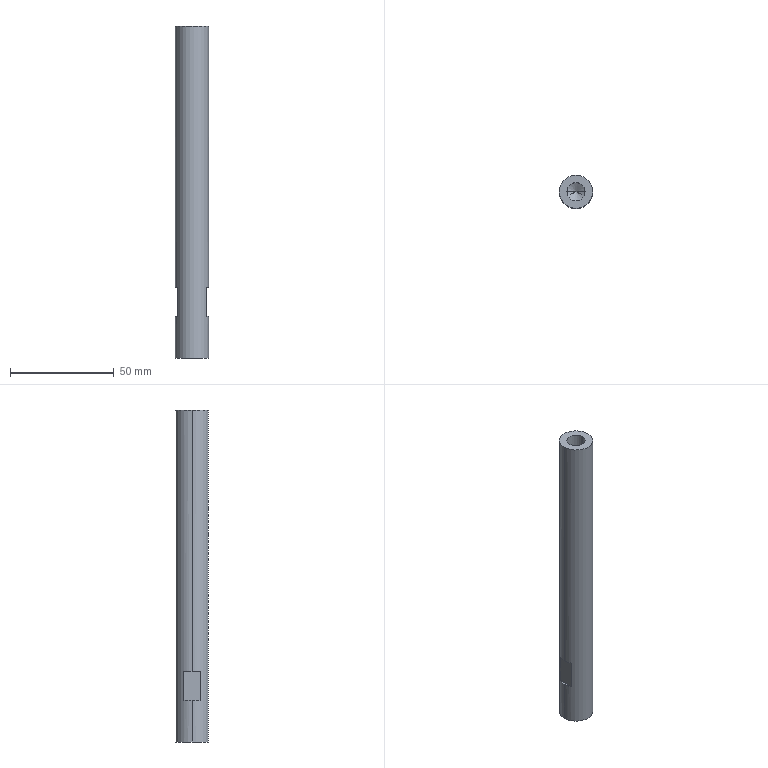Part | STEP file | Guide pillar | 1 solid | 18 faces | box 16 x 16 x 160 mm | volume 28723 mm3 | plane 8 | cylinder 6 | cone 4 | commonest cylinder face diameters 8.8 x4 16 x2
STEP:
#1=CARTESIAN_POINT('',(0.,0.,0.));
#2=DIRECTION('',(0.,0.,1.));
#3=DIRECTION('',(1.,0.,0.));
#4=AXIS2_PLACEMENT_3D('',#1,#2,#3);
#5=CARTESIAN_POINT('',(-4.4,0.,26.25));
#6=VERTEX_POINT('',#5);
#7=CARTESIAN_POINT('',(-4.4,0.,0.));
#8=VERTEX_POINT('',#7);
#9=CARTESIAN_POINT('',(-4.4,0.,0.));
#10=DIRECTION('',(0.,0.,-1.));
#11=VECTOR('',#10,1.);
#12=LINE('',#9,#11);
#13=CARTESIAN_POINT('',(0.,0.,0.));
#14=DIRECTION('',(0.,0.,-1.));
#15=DIRECTION('',(-1.,0.,0.));
#16=AXIS2_PLACEMENT_3D('',#13,#14,#15);
#17=CYLINDRICAL_SURFACE('',#16,4.4);
#18=CARTESIAN_POINT('',(6.283,0.));
#19=DIRECTION('',(0.,1.));
#20=VECTOR('',#19,1.);
#21=LINE('',#18,#20);
#22=(GEOMETRIC_REPRESENTATION_CONTEXT(2)PARAMETRIC_REPRESENTATION_CONTEXT()REPRESENTATION_CONTEXT('',''));
#23=DEFINITIONAL_REPRESENTATION('',(#21),#22);
#24=PCURVE('',#17,#23);
#25=CARTESIAN_POINT('',(0.,0.,0.));
#26=DIRECTION('',(0.,0.,-1.));
#27=DIRECTION('',(-1.,0.,0.));
#28=AXIS2_PLACEMENT_3D('',#25,#26,#27);
#29=CYLINDRICAL_SURFACE('',#28,4.4);
#30=CARTESIAN_POINT('',(0.,0.));
#31=DIRECTION('',(0.,1.));
#32=VECTOR('',#31,1.);
#33=LINE('',#30,#32);
#34=(GEOMETRIC_REPRESENTATION_CONTEXT(2)PARAMETRIC_REPRESENTATION_CONTEXT()REPRESENTATION_CONTEXT('',''));
#35=DEFINITIONAL_REPRESENTATION('',(#33),#34);
#36=PCURVE('',#29,#35);
#37=SURFACE_CURVE('',#12,(#24,#36),.PCURVE_S1.);
#38=EDGE_CURVE('',#6,#8,#37,.T.);
#39=ORIENTED_EDGE('',*,*,#38,.T.);
#40=CARTESIAN_POINT('',(4.4,0.,0.));
#41=VERTEX_POINT('',#40);
#42=CARTESIAN_POINT('',(0.,0.,0.));
#43=DIRECTION('',(0.,0.,-1.));
#44=DIRECTION('',(-1.,0.,0.));
#45=AXIS2_PLACEMENT_3D('',#42,#43,#44);
#46=CIRCLE('',#45,4.4);
#47=CARTESIAN_POINT('',(0.,0.));
#48=DIRECTION('',(1.,0.));
#49=VECTOR('',#48,1.);
#50=LINE('',#47,#49);
#51=(GEOMETRIC_REPRESENTATION_CONTEXT(2)PARAMETRIC_REPRESENTATION_CONTEXT()REPRESENTATION_CONTEXT('',''));
#52=DEFINITIONAL_REPRESENTATION('',(#50),#51);
#53=PCURVE('',#17,#52);
#54=CARTESIAN_POINT('',(0.,0.,0.));
#55=DIRECTION('',(0.,0.,1.));
#56=DIRECTION('',(1.,0.,0.));
#57=AXIS2_PLACEMENT_3D('',#54,#55,#56);
#58=PLANE('',#57);
#59=CARTESIAN_POINT('',(-4.4,0.));
#60=CARTESIAN_POINT('',(-4.4,7.621));
#61=CARTESIAN_POINT('',(2.2,3.811));
#62=CARTESIAN_POINT('',(8.8,0.));
#63=CARTESIAN_POINT('',(2.2,-3.811));
#64=CARTESIAN_POINT('',(-4.4,-7.621));
#65=CARTESIAN_POINT('',(-4.4,0.));
#66=(BOUNDED_CURVE()B_SPLINE_CURVE(2,(#59,#60,#61,#62,#63,#64,#65),.UNSPECIFIED.,.T.,.F.)B_SPLINE_CURVE_WITH_KNOTS((1,2,2,2,2,1),(-2.094,0.,2.094,4.189,6.283,8.378),.UNSPECIFIED.)CURVE()GEOMETRIC_REPRESENTATION_ITEM()RATIONAL_B_SPLINE_CURVE((1.,0.5,1.,0.5,1.,0.5,1.))REPRESENTATION_ITEM(''));
#67=(GEOMETRIC_REPRESENTATION_CONTEXT(2)PARAMETRIC_REPRESENTATION_CONTEXT()REPRESENTATION_CONTEXT('',''));
#68=DEFINITIONAL_REPRESENTATION('',(#66),#67);
#69=PCURVE('',#58,#68);
#70=SURFACE_CURVE('',#46,(#53,#69),.PCURVE_S1.);
#71=EDGE_CURVE('',#41,#8,#70,.T.);
#72=ORIENTED_EDGE('',*,*,#71,.F.);
#73=CARTESIAN_POINT('',(4.4,0.,26.25));
#74=VERTEX_POINT('',#73);
#75=CARTESIAN_POINT('',(4.4,0.,0.));
#76=DIRECTION('',(0.,0.,-1.));
#77=VECTOR('',#76,1.);
#78=LINE('',#75,#77);
#79=CARTESIAN_POINT('',(3.142,0.));
#80=DIRECTION('',(0.,1.));
#81=VECTOR('',#80,1.);
#82=LINE('',#79,#81);
#83=(GEOMETRIC_REPRESENTATION_CONTEXT(2)PARAMETRIC_REPRESENTATION_CONTEXT()REPRESENTATION_CONTEXT('',''));
#84=DEFINITIONAL_REPRESENTATION('',(#82),#83);
#85=PCURVE('',#17,#84);
#86=CARTESIAN_POINT('',(3.142,0.));
#87=DIRECTION('',(0.,1.));
#88=VECTOR('',#87,1.);
#89=LINE('',#86,#88);
#90=(GEOMETRIC_REPRESENTATION_CONTEXT(2)PARAMETRIC_REPRESENTATION_CONTEXT()REPRESENTATION_CONTEXT('',''));
#91=DEFINITIONAL_REPRESENTATION('',(#89),#90);
#92=PCURVE('',#29,#91);
#93=SURFACE_CURVE('',#78,(#85,#92),.PCURVE_S1.);
#94=EDGE_CURVE('',#74,#41,#93,.T.);
#95=ORIENTED_EDGE('',*,*,#94,.F.);
#96=CARTESIAN_POINT('',(0.,0.,26.25));
#97=DIRECTION('',(0.,0.,-1.));
#98=DIRECTION('',(-1.,0.,0.));
#99=AXIS2_PLACEMENT_3D('',#96,#97,#98);
#100=CIRCLE('',#99,4.4);
#101=CARTESIAN_POINT('',(0.,-26.25));
#102=DIRECTION('',(1.,0.));
#103=VECTOR('',#102,1.);
#104=LINE('',#101,#103);
#105=(GEOMETRIC_REPRESENTATION_CONTEXT(2)PARAMETRIC_REPRESENTATION_CONTEXT()REPRESENTATION_CONTEXT('',''));
#106=DEFINITIONAL_REPRESENTATION('',(#104),#105);
#107=PCURVE('',#17,#106);
#108=CARTESIAN_POINT('',(0.,0.,26.25));
#109=DIRECTION('',(0.,0.,-1.));
#110=DIRECTION('',(-1.,0.,0.));
#111=AXIS2_PLACEMENT_3D('',#108,#109,#110);
#112=CONICAL_SURFACE('',#111,4.4,1.03);
#113=CARTESIAN_POINT('',(0.,0.));
#114=DIRECTION('',(1.,0.));
#115=VECTOR('',#114,1.);
#116=LINE('',#113,#115);
#117=(GEOMETRIC_REPRESENTATION_CONTEXT(2)PARAMETRIC_REPRESENTATION_CONTEXT()REPRESENTATION_CONTEXT('',''));
#118=DEFINITIONAL_REPRESENTATION('',(#116),#117);
#119=PCURVE('',#112,#118);
#120=SURFACE_CURVE('',#100,(#107,#119),.PCURVE_S1.);
#121=EDGE_CURVE('',#74,#6,#120,.T.);
#122=ORIENTED_EDGE('',*,*,#121,.T.);
#123=EDGE_LOOP('',(#39,#72,#95,#122));
#124=FACE_BOUND('',#123,.F.);
#125=ADVANCED_FACE('',(#124),#17,.F.);
#126=ORIENTED_EDGE('',*,*,#121,.F.);
#127=CARTESIAN_POINT('',(0.,0.,28.894));
#128=VERTEX_POINT('',#127);
#129=CARTESIAN_POINT('',(4.4,0.,26.25));
#130=DIRECTION('',(0.8572,0.,-0.515));
#131=VECTOR('',#130,1.);
#132=LINE('',#129,#131);
#133=CARTESIAN_POINT('',(3.142,0.));
#134=DIRECTION('',(0.,1.));
#135=VECTOR('',#134,1.);
#136=LINE('',#133,#135);
#137=(GEOMETRIC_REPRESENTATION_CONTEXT(2)PARAMETRIC_REPRESENTATION_CONTEXT()REPRESENTATION_CONTEXT('',''));
#138=DEFINITIONAL_REPRESENTATION('',(#136),#137);
#139=PCURVE('',#112,#138);
#140=CARTESIAN_POINT('',(0.,0.,26.25));
#141=DIRECTION('',(0.,0.,-1.));
#142=DIRECTION('',(-1.,0.,0.));
#143=AXIS2_PLACEMENT_3D('',#140,#141,#142);
#144=CONICAL_SURFACE('',#143,4.4,1.03);
#145=CARTESIAN_POINT('',(3.142,0.));
#146=DIRECTION('',(0.,1.));
#147=VECTOR('',#146,1.);
#148=LINE('',#145,#147);
#149=(GEOMETRIC_REPRESENTATION_CONTEXT(2)PARAMETRIC_REPRESENTATION_CONTEXT()REPRESENTATION_CONTEXT('',''));
#150=DEFINITIONAL_REPRESENTATION('',(#148),#149);
#151=PCURVE('',#144,#150);
#152=SURFACE_CURVE('',#132,(#139,#151),.PCURVE_S1.);
#153=EDGE_CURVE('',#128,#74,#152,.T.);
#154=ORIENTED_EDGE('',*,*,#153,.F.);
#155=CARTESIAN_POINT('',(-4.4,0.,26.25));
#156=DIRECTION('',(-0.8572,0.,-0.515));
#157=VECTOR('',#156,1.);
#158=LINE('',#155,#157);
#159=CARTESIAN_POINT('',(6.283,0.));
#160=DIRECTION('',(0.,1.));
#161=VECTOR('',#160,1.);
#162=LINE('',#159,#161);
#163=(GEOMETRIC_REPRESENTATION_CONTEXT(2)PARAMETRIC_REPRESENTATION_CONTEXT()REPRESENTATION_CONTEXT('',''));
#164=DEFINITIONAL_REPRESENTATION('',(#162),#163);
#165=PCURVE('',#112,#164);
#166=CARTESIAN_POINT('',(0.,0.));
#167=DIRECTION('',(0.,1.));
#168=VECTOR('',#167,1.);
#169=LINE('',#166,#168);
#170=(GEOMETRIC_REPRESENTATION_CONTEXT(2)PARAMETRIC_REPRESENTATION_CONTEXT()REPRESENTATION_CONTEXT('',''));
#171=DEFINITIONAL_REPRESENTATION('',(#169),#170);
#172=PCURVE('',#144,#171);
#173=SURFACE_CURVE('',#158,(#165,#172),.PCURVE_S1.);
#174=EDGE_CURVE('',#128,#6,#173,.T.);
#175=ORIENTED_EDGE('',*,*,#174,.T.);
#176=EDGE_LOOP('',(#126,#154,#175));
#177=FACE_BOUND('',#176,.F.);
#178=ADVANCED_FACE('',(#177),#112,.F.);
#179=CARTESIAN_POINT('',(4.4,0.,133.75));
#180=VERTEX_POINT('',#179);
#181=CARTESIAN_POINT('',(4.4,0.,160.));
#182=VERTEX_POINT('',#181);
#183=CARTESIAN_POINT('',(4.4,0.,160.));
#184=DIRECTION('',(0.,0.,1.));
#185=VECTOR('',#184,1.);
#186=LINE('',#183,#185);
#187=CARTESIAN_POINT('',(0.,0.,160.));
#188=DIRECTION('',(0.,0.,1.));
#189=DIRECTION('',(1.,0.,0.));
#190=AXIS2_PLACEMENT_3D('',#187,#188,#189);
#191=CYLINDRICAL_SURFACE('',#190,4.4);
#192=CARTESIAN_POINT('',(6.283,0.));
#193=DIRECTION('',(0.,1.));
#194=VECTOR('',#193,1.);
#195=LINE('',#192,#194);
#196=(GEOMETRIC_REPRESENTATION_CONTEXT(2)PARAMETRIC_REPRESENTATION_CONTEXT()REPRESENTATION_CONTEXT('',''));
#197=DEFINITIONAL_REPRESENTATION('',(#195),#196);
#198=PCURVE('',#191,#197);
#199=CARTESIAN_POINT('',(0.,0.,160.));
#200=DIRECTION('',(0.,0.,1.));
#201=DIRECTION('',(1.,0.,0.));
#202=AXIS2_PLACEMENT_3D('',#199,#200,#201);
#203=CYLINDRICAL_SURFACE('',#202,4.4);
#204=CARTESIAN_POINT('',(0.,0.));
#205=DIRECTION('',(0.,1.));
#206=VECTOR('',#205,1.);
#207=LINE('',#204,#206);
#208=(GEOMETRIC_REPRESENTATION_CONTEXT(2)PARAMETRIC_REPRESENTATION_CONTEXT()REPRESENTATION_CONTEXT('',''));
#209=DEFINITIONAL_REPRESENTATION('',(#207),#208);
#210=PCURVE('',#203,#209);
#211=SURFACE_CURVE('',#186,(#198,#210),.PCURVE_S1.);
#212=EDGE_CURVE('',#180,#182,#211,.T.);
#213=ORIENTED_EDGE('',*,*,#212,.T.);
#214=CARTESIAN_POINT('',(-4.4,0.,160.));
#215=VERTEX_POINT('',#214);
#216=CARTESIAN_POINT('',(0.,0.,160.));
#217=DIRECTION('',(0.,0.,1.));
#218=DIRECTION('',(1.,0.,0.));
#219=AXIS2_PLACEMENT_3D('',#216,#217,#218);
#220=CIRCLE('',#219,4.4);
#221=CARTESIAN_POINT('',(0.,0.));
#222=DIRECTION('',(1.,0.));
#223=VECTOR('',#222,1.);
#224=LINE('',#221,#223);
#225=(GEOMETRIC_REPRESENTATION_CONTEXT(2)PARAMETRIC_REPRESENTATION_CONTEXT()REPRESENTATION_CONTEXT('',''));
#226=DEFINITIONAL_REPRESENTATION('',(#224),#225);
#227=PCURVE('',#191,#226);
#228=CARTESIAN_POINT('',(0.,0.,160.));
#229=DIRECTION('',(0.,0.,1.));
#230=DIRECTION('',(1.,0.,0.));
#231=AXIS2_PLACEMENT_3D('',#228,#229,#230);
#232=PLANE('',#231);
#233=CARTESIAN_POINT('',(0.,0.));
#234=DIRECTION('',(1.,0.));
#235=AXIS2_PLACEMENT_2D('',#233,#234);
#236=CIRCLE('',#235,4.4);
#237=(GEOMETRIC_REPRESENTATION_CONTEXT(2)PARAMETRIC_REPRESENTATION_CONTEXT()REPRESENTATION_CONTEXT('',''));
#238=DEFINITIONAL_REPRESENTATION('',(#236),#237);
#239=PCURVE('',#232,#238);
#240=SURFACE_CURVE('',#220,(#227,#239),.PCURVE_S1.);
#241=EDGE_CURVE('',#215,#182,#240,.T.);
#242=ORIENTED_EDGE('',*,*,#241,.F.);
#243=CARTESIAN_POINT('',(-4.4,0.,133.75));
#244=VERTEX_POINT('',#243);
#245=CARTESIAN_POINT('',(-4.4,0.,160.));
#246=DIRECTION('',(0.,0.,1.));
#247=VECTOR('',#246,1.);
#248=LINE('',#245,#247);
#249=CARTESIAN_POINT('',(3.142,0.));
#250=DIRECTION('',(0.,1.));
#251=VECTOR('',#250,1.);
#252=LINE('',#249,#251);
#253=(GEOMETRIC_REPRESENTATION_CONTEXT(2)PARAMETRIC_REPRESENTATION_CONTEXT()REPRESENTATION_CONTEXT('',''));
#254=DEFINITIONAL_REPRESENTATION('',(#252),#253);
#255=PCURVE('',#191,#254);
#256=CARTESIAN_POINT('',(3.142,0.));
#257=DIRECTION('',(0.,1.));
#258=VECTOR('',#257,1.);
#259=LINE('',#256,#258);
#260=(GEOMETRIC_REPRESENTATION_CONTEXT(2)PARAMETRIC_REPRESENTATION_CONTEXT()REPRESENTATION_CONTEXT('',''));
#261=DEFINITIONAL_REPRESENTATION('',(#259),#260);
#262=PCURVE('',#203,#261);
#263=SURFACE_CURVE('',#248,(#255,#262),.PCURVE_S1.);
#264=EDGE_CURVE('',#244,#215,#263,.T.);
#265=ORIENTED_EDGE('',*,*,#264,.F.);
#266=CARTESIAN_POINT('',(0.,0.,133.75));
#267=DIRECTION('',(0.,0.,1.));
#268=DIRECTION('',(1.,0.,0.));
#269=AXIS2_PLACEMENT_3D('',#266,#267,#268);
#270=CIRCLE('',#269,4.4);
#271=CARTESIAN_POINT('',(0.,-26.25));
#272=DIRECTION('',(1.,0.));
#273=VECTOR('',#272,1.);
#274=LINE('',#271,#273);
#275=(GEOMETRIC_REPRESENTATION_CONTEXT(2)PARAMETRIC_REPRESENTATION_CONTEXT()REPRESENTATION_CONTEXT('',''));
#276=DEFINITIONAL_REPRESENTATION('',(#274),#275);
#277=PCURVE('',#191,#276);
#278=CARTESIAN_POINT('',(0.,0.,133.75));
#279=DIRECTION('',(0.,0.,1.));
#280=DIRECTION('',(1.,0.,0.));
#281=AXIS2_PLACEMENT_3D('',#278,#279,#280);
#282=CONICAL_SURFACE('',#281,4.4,1.03);
#283=CARTESIAN_POINT('',(0.,0.));
#284=DIRECTION('',(1.,0.));
#285=VECTOR('',#284,1.);
#286=LINE('',#283,#285);
#287=(GEOMETRIC_REPRESENTATION_CONTEXT(2)PARAMETRIC_REPRESENTATION_CONTEXT()REPRESENTATION_CONTEXT('',''));
#288=DEFINITIONAL_REPRESENTATION('',(#286),#287);
#289=PCURVE('',#282,#288);
#290=SURFACE_CURVE('',#270,(#277,#289),.PCURVE_S1.);
#291=EDGE_CURVE('',#244,#180,#290,.T.);
#292=ORIENTED_EDGE('',*,*,#291,.T.);
#293=EDGE_LOOP('',(#213,#242,#265,#292));
#294=FACE_BOUND('',#293,.F.);
#295=ADVANCED_FACE('',(#294),#191,.F.);
#296=ORIENTED_EDGE('',*,*,#291,.F.);
#297=CARTESIAN_POINT('',(0.,0.,131.106));
#298=VERTEX_POINT('',#297);
#299=CARTESIAN_POINT('',(-4.4,0.,133.75));
#300=DIRECTION('',(-0.8572,0.,0.515));
#301=VECTOR('',#300,1.);
#302=LINE('',#299,#301);
#303=CARTESIAN_POINT('',(3.142,-2.644));
#304=CARTESIAN_POINT('',(3.142,-2.604));
#305=CARTESIAN_POINT('',(3.142,-2.524));
#306=CARTESIAN_POINT('',(3.142,-2.403));
#307=CARTESIAN_POINT('',(3.142,-2.283));
#308=CARTESIAN_POINT('',(3.142,-2.163));
#309=CARTESIAN_POINT('',(3.142,-2.043));
#310=CARTESIAN_POINT('',(3.142,-1.923));
#311=CARTESIAN_POINT('',(3.142,-1.803));
#312=CARTESIAN_POINT('',(3.142,-1.682));
#313=CARTESIAN_POINT('',(3.142,-1.562));
#314=CARTESIAN_POINT('',(3.142,-1.442));
#315=CARTESIAN_POINT('',(3.142,-1.322));
#316=CARTESIAN_POINT('',(3.142,-1.202));
#317=CARTESIAN_POINT('',(3.142,-1.082));
#318=CARTESIAN_POINT('',(3.142,-0.9614));
#319=CARTESIAN_POINT('',(3.142,-0.8412));
#320=CARTESIAN_POINT('',(3.142,-0.721));
#321=CARTESIAN_POINT('',(3.142,-0.6009));
#322=CARTESIAN_POINT('',(3.142,-0.4807));
#323=CARTESIAN_POINT('',(3.142,-0.3605));
#324=CARTESIAN_POINT('',(3.142,-0.2403));
#325=CARTESIAN_POINT('',(3.142,-0.1202));
#326=CARTESIAN_POINT('',(3.142,-0.04006));
#327=CARTESIAN_POINT('',(3.142,0.));
#328=B_SPLINE_CURVE_WITH_KNOTS('',3,(#303,#304,#305,#306,#307,#308,#309,#310,#311,#312,#313,#314,#315,#316,#317,#318,#319,#320,#321,#322,#323,#324,#325,#326,#327),.UNSPECIFIED.,.F.,.F.,(4,1,1,1,1,1,1,1,1,1,1,1,1,1,1,1,1,1,1,1,1,1,4),(-5.133,-4.9,-4.667,-4.433,-4.2,-3.967,-3.733,-3.5,-3.267,-3.033,-2.8,-2.567,-2.333,-2.1,-1.867,-1.633,-1.4,-1.167,-0.9333,-0.7,-0.4667,-0.2333,0.),.UNSPECIFIED.);
#329=(GEOMETRIC_REPRESENTATION_CONTEXT(2)PARAMETRIC_REPRESENTATION_CONTEXT()REPRESENTATION_CONTEXT('',''));
#330=DEFINITIONAL_REPRESENTATION('',(#328),#329);
#331=PCURVE('',#282,#330);
#332=CARTESIAN_POINT('',(0.,0.,133.75));
#333=DIRECTION('',(0.,0.,1.));
#334=DIRECTION('',(1.,0.,0.));
#335=AXIS2_PLACEMENT_3D('',#332,#333,#334);
#336=CONICAL_SURFACE('',#335,4.4,1.03);
#337=CARTESIAN_POINT('',(3.142,-2.644));
#338=CARTESIAN_POINT('',(3.142,-2.604));
#339=CARTESIAN_POINT('',(3.142,-2.524));
#340=CARTESIAN_POINT('',(3.142,-2.403));
#341=CARTESIAN_POINT('',(3.142,-2.283));
#342=CARTESIAN_POINT('',(3.142,-2.163));
#343=CARTESIAN_POINT('',(3.142,-2.043));
#344=CARTESIAN_POINT('',(3.142,-1.923));
#345=CARTESIAN_POINT('',(3.142,-1.803));
#346=CARTESIAN_POINT('',(3.142,-1.682));
#347=CARTESIAN_POINT('',(3.142,-1.562));
#348=CARTESIAN_POINT('',(3.142,-1.442));
#349=CARTESIAN_POINT('',(3.142,-1.322));
#350=CARTESIAN_POINT('',(3.142,-1.202));
#351=CARTESIAN_POINT('',(3.142,-1.082));
#352=CARTESIAN_POINT('',(3.142,-0.9614));
#353=CARTESIAN_POINT('',(3.142,-0.8412));
#354=CARTESIAN_POINT('',(3.142,-0.721));
#355=CARTESIAN_POINT('',(3.142,-0.6009));
#356=CARTESIAN_POINT('',(3.142,-0.4807));
#357=CARTESIAN_POINT('',(3.142,-0.3605));
#358=CARTESIAN_POINT('',(3.142,-0.2403));
#359=CARTESIAN_POINT('',(3.142,-0.1202));
#360=CARTESIAN_POINT('',(3.142,-0.04006));
#361=CARTESIAN_POINT('',(3.142,0.));
#362=B_SPLINE_CURVE_WITH_KNOTS('',3,(#337,#338,#339,#340,#341,#342,#343,#344,#345,#346,#347,#348,#349,#350,#351,#352,#353,#354,#355,#356,#357,#358,#359,#360,#361),.UNSPECIFIED.,.F.,.F.,(4,1,1,1,1,1,1,1,1,1,1,1,1,1,1,1,1,1,1,1,1,1,4),(-5.133,-4.9,-4.667,-4.433,-4.2,-3.967,-3.733,-3.5,-3.267,-3.033,-2.8,-2.567,-2.333,-2.1,-1.867,-1.633,-1.4,-1.167,-0.9333,-0.7,-0.4667,-0.2333,0.),.UNSPECIFIED.);
#363=(GEOMETRIC_REPRESENTATION_CONTEXT(2)PARAMETRIC_REPRESENTATION_CONTEXT()REPRESENTATION_CONTEXT('',''));
#364=DEFINITIONAL_REPRESENTATION('',(#362),#363);
#365=PCURVE('',#336,#364);
#366=SURFACE_CURVE('',#302,(#331,#365),.PCURVE_S1.);
#367=EDGE_CURVE('',#298,#244,#366,.T.);
#368=ORIENTED_EDGE('',*,*,#367,.F.);
#369=CARTESIAN_POINT('',(4.4,0.,133.75));
#370=DIRECTION('',(0.8572,0.,0.515));
#371=VECTOR('',#370,1.);
#372=LINE('',#369,#371);
#373=CARTESIAN_POINT('',(6.283,0.));
#374=DIRECTION('',(0.,1.));
#375=VECTOR('',#374,1.);
#376=LINE('',#373,#375);
#377=(GEOMETRIC_REPRESENTATION_CONTEXT(2)PARAMETRIC_REPRESENTATION_CONTEXT()REPRESENTATION_CONTEXT('',''));
#378=DEFINITIONAL_REPRESENTATION('',(#376),#377);
#379=PCURVE('',#282,#378);
#380=CARTESIAN_POINT('',(0.,0.));
#381=DIRECTION('',(0.,1.));
#382=VECTOR('',#381,1.);
#383=LINE('',#380,#382);
#384=(GEOMETRIC_REPRESENTATION_CONTEXT(2)PARAMETRIC_REPRESENTATION_CONTEXT()REPRESENTATION_CONTEXT('',''));
#385=DEFINITIONAL_REPRESENTATION('',(#383),#384);
#386=PCURVE('',#336,#385);
#387=SURFACE_CURVE('',#372,(#379,#386),.PCURVE_S1.);
#388=EDGE_CURVE('',#298,#180,#387,.T.);
#389=ORIENTED_EDGE('',*,*,#388,.T.);
#390=EDGE_LOOP('',(#296,#368,#389));
#391=FACE_BOUND('',#390,.F.);
#392=ADVANCED_FACE('',(#391),#282,.F.);
#393=CARTESIAN_POINT('',(8.,0.,160.));
#394=VERTEX_POINT('',#393);
#395=CARTESIAN_POINT('',(-8.,0.,160.));
#396=VERTEX_POINT('',#395);
#397=CARTESIAN_POINT('',(0.,0.,160.));
#398=DIRECTION('',(0.,0.,1.));
#399=DIRECTION('',(1.,0.,0.));
#400=AXIS2_PLACEMENT_3D('',#397,#398,#399);
#401=CIRCLE('',#400,8.);
#402=CARTESIAN_POINT('',(0.,0.,160.));
#403=DIRECTION('',(0.,0.,-1.));
#404=DIRECTION('',(-1.,0.,0.));
#405=AXIS2_PLACEMENT_3D('',#402,#403,#404);
#406=CYLINDRICAL_SURFACE('',#405,8.);
#407=CARTESIAN_POINT('',(3.142,0.));
#408=DIRECTION('',(-1.,0.));
#409=VECTOR('',#408,1.);
#410=LINE('',#407,#409);
#411=(GEOMETRIC_REPRESENTATION_CONTEXT(2)PARAMETRIC_REPRESENTATION_CONTEXT()REPRESENTATION_CONTEXT('',''));
#412=DEFINITIONAL_REPRESENTATION('',(#410),#411);
#413=PCURVE('',#406,#412);
#414=CARTESIAN_POINT('',(0.,0.));
#415=DIRECTION('',(1.,0.));
#416=AXIS2_PLACEMENT_2D('',#414,#415);
#417=CIRCLE('',#416,8.);
#418=(GEOMETRIC_REPRESENTATION_CONTEXT(2)PARAMETRIC_REPRESENTATION_CONTEXT()REPRESENTATION_CONTEXT('',''));
#419=DEFINITIONAL_REPRESENTATION('',(#417),#418);
#420=PCURVE('',#232,#419);
#421=SURFACE_CURVE('',#401,(#413,#420),.PCURVE_S1.);
#422=EDGE_CURVE('',#394,#396,#421,.T.);
#423=ORIENTED_EDGE('',*,*,#422,.F.);
#424=CARTESIAN_POINT('',(8.,0.,34.));
#425=VERTEX_POINT('',#424);
#426=CARTESIAN_POINT('',(8.,0.,160.));
#427=DIRECTION('',(0.,0.,-1.));
#428=VECTOR('',#427,1.);
#429=LINE('',#426,#428);
#430=CARTESIAN_POINT('',(3.142,0.));
#431=DIRECTION('',(0.,1.));
#432=VECTOR('',#431,1.);
#433=LINE('',#430,#432);
#434=(GEOMETRIC_REPRESENTATION_CONTEXT(2)PARAMETRIC_REPRESENTATION_CONTEXT()REPRESENTATION_CONTEXT('',''));
#435=DEFINITIONAL_REPRESENTATION('',(#433),#434);
#436=PCURVE('',#406,#435);
#437=CARTESIAN_POINT('',(0.,0.,160.));
#438=DIRECTION('',(0.,0.,-1.));
#439=DIRECTION('',(-1.,0.,0.));
#440=AXIS2_PLACEMENT_3D('',#437,#438,#439);
#441=CYLINDRICAL_SURFACE('',#440,8.);
#442=CARTESIAN_POINT('',(3.142,0.));
#443=DIRECTION('',(0.,1.));
#444=VECTOR('',#443,1.);
#445=LINE('',#442,#444);
#446=(GEOMETRIC_REPRESENTATION_CONTEXT(2)PARAMETRIC_REPRESENTATION_CONTEXT()REPRESENTATION_CONTEXT('',''));
#447=DEFINITIONAL_REPRESENTATION('',(#445),#446);
#448=PCURVE('',#441,#447);
#449=SURFACE_CURVE('',#429,(#436,#448),.PCURVE_S1.);
#450=EDGE_CURVE('',#394,#425,#449,.T.);
#451=ORIENTED_EDGE('',*,*,#450,.T.);
#452=CARTESIAN_POINT('',(7.,3.873,34.));
#453=VERTEX_POINT('',#452);
#454=CARTESIAN_POINT('',(0.,0.,34.));
#455=DIRECTION('',(0.,0.,1.));
#456=DIRECTION('',(1.,0.,0.));
#457=AXIS2_PLACEMENT_3D('',#454,#455,#456);
#458=CIRCLE('',#457,8.);
#459=CARTESIAN_POINT('',(3.142,126.));
#460=DIRECTION('',(-1.,0.));
#461=VECTOR('',#460,1.);
#462=LINE('',#459,#461);
#463=(GEOMETRIC_REPRESENTATION_CONTEXT(2)PARAMETRIC_REPRESENTATION_CONTEXT()REPRESENTATION_CONTEXT('',''));
#464=DEFINITIONAL_REPRESENTATION('',(#462),#463);
#465=PCURVE('',#406,#464);
#466=CARTESIAN_POINT('',(7.,-8.391,34.));
#467=DIRECTION('',(0.,0.,1.));
#468=DIRECTION('',(1.,0.,0.));
#469=AXIS2_PLACEMENT_3D('',#466,#467,#468);
#470=PLANE('',#469);
#471=CARTESIAN_POINT('',(-7.,8.391));
#472=DIRECTION('',(1.,0.));
#473=AXIS2_PLACEMENT_2D('',#471,#472);
#474=CIRCLE('',#473,8.);
#475=(GEOMETRIC_REPRESENTATION_CONTEXT(2)PARAMETRIC_REPRESENTATION_CONTEXT()REPRESENTATION_CONTEXT('',''));
#476=DEFINITIONAL_REPRESENTATION('',(#474),#475);
#477=PCURVE('',#470,#476);
#478=SURFACE_CURVE('',#458,(#465,#477),.PCURVE_S1.);
#479=EDGE_CURVE('',#425,#453,#478,.T.);
#480=ORIENTED_EDGE('',*,*,#479,.T.);
#481=CARTESIAN_POINT('',(7.,3.873,20.));
#482=VERTEX_POINT('',#481);
#483=CARTESIAN_POINT('',(7.,3.873,160.));
#484=DIRECTION('',(0.,0.,-1.));
#485=VECTOR('',#484,1.);
#486=LINE('',#483,#485);
#487=CARTESIAN_POINT('',(2.636,0.));
#488=DIRECTION('',(0.,1.));
#489=VECTOR('',#488,1.);
#490=LINE('',#487,#489);
#491=(GEOMETRIC_REPRESENTATION_CONTEXT(2)PARAMETRIC_REPRESENTATION_CONTEXT()REPRESENTATION_CONTEXT('',''));
#492=DEFINITIONAL_REPRESENTATION('',(#490),#491);
#493=PCURVE('',#406,#492);
#494=CARTESIAN_POINT('',(7.,9.789,34.));
#495=DIRECTION('',(-1.,0.,0.));
#496=DIRECTION('',(0.,-1.,0.));
#497=AXIS2_PLACEMENT_3D('',#494,#495,#496);
#498=PLANE('',#497);
#499=CARTESIAN_POINT('',(5.916,126.));
#500=DIRECTION('',(0.,-1.));
#501=VECTOR('',#500,1.);
#502=LINE('',#499,#501);
#503=(GEOMETRIC_REPRESENTATION_CONTEXT(2)PARAMETRIC_REPRESENTATION_CONTEXT()REPRESENTATION_CONTEXT('',''));
#504=DEFINITIONAL_REPRESENTATION('',(#502),#503);
#505=PCURVE('',#498,#504);
#506=SURFACE_CURVE('',#486,(#493,#505),.PCURVE_S1.);
#507=EDGE_CURVE('',#453,#482,#506,.T.);
#508=ORIENTED_EDGE('',*,*,#507,.T.);
#509=CARTESIAN_POINT('',(8.,0.,20.));
#510=VERTEX_POINT('',#509);
#511=CARTESIAN_POINT('',(0.,0.,20.));
#512=DIRECTION('',(0.,0.,1.));
#513=DIRECTION('',(1.,0.,0.));
#514=AXIS2_PLACEMENT_3D('',#511,#512,#513);
#515=CIRCLE('',#514,8.);
#516=CARTESIAN_POINT('',(3.142,140.));
#517=DIRECTION('',(-1.,0.));
#518=VECTOR('',#517,1.);
#519=LINE('',#516,#518);
#520=(GEOMETRIC_REPRESENTATION_CONTEXT(2)PARAMETRIC_REPRESENTATION_CONTEXT()REPRESENTATION_CONTEXT('',''));
#521=DEFINITIONAL_REPRESENTATION('',(#519),#520);
#522=PCURVE('',#406,#521);
#523=CARTESIAN_POINT('',(7.,-8.391,20.));
#524=DIRECTION('',(0.,0.,1.));
#525=DIRECTION('',(1.,0.,0.));
#526=AXIS2_PLACEMENT_3D('',#523,#524,#525);
#527=PLANE('',#526);
#528=CARTESIAN_POINT('',(-7.,8.391));
#529=DIRECTION('',(1.,0.));
#530=AXIS2_PLACEMENT_2D('',#528,#529);
#531=CIRCLE('',#530,8.);
#532=(GEOMETRIC_REPRESENTATION_CONTEXT(2)PARAMETRIC_REPRESENTATION_CONTEXT()REPRESENTATION_CONTEXT('',''));
#533=DEFINITIONAL_REPRESENTATION('',(#531),#532);
#534=PCURVE('',#527,#533);
#535=SURFACE_CURVE('',#515,(#522,#534),.PCURVE_S1.);
#536=EDGE_CURVE('',#510,#482,#535,.T.);
#537=ORIENTED_EDGE('',*,*,#536,.F.);
#538=CARTESIAN_POINT('',(8.,0.,0.));
#539=VERTEX_POINT('',#538);
#540=CARTESIAN_POINT('',(8.,0.,160.));
#541=DIRECTION('',(0.,0.,-1.));
#542=VECTOR('',#541,1.);
#543=LINE('',#540,#542);
#544=CARTESIAN_POINT('',(3.142,0.));
#545=DIRECTION('',(0.,1.));
#546=VECTOR('',#545,1.);
#547=LINE('',#544,#546);
#548=(GEOMETRIC_REPRESENTATION_CONTEXT(2)PARAMETRIC_REPRESENTATION_CONTEXT()REPRESENTATION_CONTEXT('',''));
#549=DEFINITIONAL_REPRESENTATION('',(#547),#548);
#550=PCURVE('',#406,#549);
#551=CARTESIAN_POINT('',(3.142,0.));
#552=DIRECTION('',(0.,1.));
#553=VECTOR('',#552,1.);
#554=LINE('',#551,#553);
#555=(GEOMETRIC_REPRESENTATION_CONTEXT(2)PARAMETRIC_REPRESENTATION_CONTEXT()REPRESENTATION_CONTEXT('',''));
#556=DEFINITIONAL_REPRESENTATION('',(#554),#555);
#557=PCURVE('',#441,#556);
#558=SURFACE_CURVE('',#543,(#550,#557),.PCURVE_S1.);
#559=EDGE_CURVE('',#510,#539,#558,.T.);
#560=ORIENTED_EDGE('',*,*,#559,.T.);
#561=CARTESIAN_POINT('',(-8.,0.,0.));
#562=VERTEX_POINT('',#561);
#563=CARTESIAN_POINT('',(0.,0.,0.));
#564=DIRECTION('',(0.,0.,1.));
#565=DIRECTION('',(1.,0.,0.));
#566=AXIS2_PLACEMENT_3D('',#563,#564,#565);
#567=CIRCLE('',#566,8.);
#568=CARTESIAN_POINT('',(3.142,160.));
#569=DIRECTION('',(-1.,0.));
#570=VECTOR('',#569,1.);
#571=LINE('',#568,#570);
#572=(GEOMETRIC_REPRESENTATION_CONTEXT(2)PARAMETRIC_REPRESENTATION_CONTEXT()REPRESENTATION_CONTEXT('',''));
#573=DEFINITIONAL_REPRESENTATION('',(#571),#572);
#574=PCURVE('',#406,#573);
#575=CARTESIAN_POINT('',(0.,0.));
#576=DIRECTION('',(1.,0.));
#577=AXIS2_PLACEMENT_2D('',#575,#576);
#578=CIRCLE('',#577,8.);
#579=(GEOMETRIC_REPRESENTATION_CONTEXT(2)PARAMETRIC_REPRESENTATION_CONTEXT()REPRESENTATION_CONTEXT('',''));
#580=DEFINITIONAL_REPRESENTATION('',(#578),#579);
#581=PCURVE('',#58,#580);
#582=SURFACE_CURVE('',#567,(#574,#581),.PCURVE_S1.);
#583=EDGE_CURVE('',#539,#562,#582,.T.);
#584=ORIENTED_EDGE('',*,*,#583,.T.);
#585=CARTESIAN_POINT('',(-8.,0.,20.));
#586=VERTEX_POINT('',#585);
#587=CARTESIAN_POINT('',(-8.,0.,160.));
#588=DIRECTION('',(0.,0.,-1.));
#589=VECTOR('',#588,1.);
#590=LINE('',#587,#589);
#591=CARTESIAN_POINT('',(0.,0.));
#592=DIRECTION('',(0.,1.));
#593=VECTOR('',#592,1.);
#594=LINE('',#591,#593);
#595=(GEOMETRIC_REPRESENTATION_CONTEXT(2)PARAMETRIC_REPRESENTATION_CONTEXT()REPRESENTATION_CONTEXT('',''));
#596=DEFINITIONAL_REPRESENTATION('',(#594),#595);
#597=PCURVE('',#406,#596);
#598=CARTESIAN_POINT('',(6.283,0.));
#599=DIRECTION('',(0.,1.));
#600=VECTOR('',#599,1.);
#601=LINE('',#598,#600);
#602=(GEOMETRIC_REPRESENTATION_CONTEXT(2)PARAMETRIC_REPRESENTATION_CONTEXT()REPRESENTATION_CONTEXT('',''));
#603=DEFINITIONAL_REPRESENTATION('',(#601),#602);
#604=PCURVE('',#441,#603);
#605=SURFACE_CURVE('',#590,(#597,#604),.PCURVE_S1.);
#606=EDGE_CURVE('',#586,#562,#605,.T.);
#607=ORIENTED_EDGE('',*,*,#606,.F.);
#608=CARTESIAN_POINT('',(-7.,3.873,20.));
#609=VERTEX_POINT('',#608);
#610=CARTESIAN_POINT('',(0.,0.,20.));
#611=DIRECTION('',(0.,0.,1.));
#612=DIRECTION('',(1.,0.,0.));
#613=AXIS2_PLACEMENT_3D('',#610,#611,#612);
#614=CIRCLE('',#613,8.);
#615=CARTESIAN_POINT('',(3.142,140.));
#616=DIRECTION('',(-1.,0.));
#617=VECTOR('',#616,1.);
#618=LINE('',#615,#617);
#619=(GEOMETRIC_REPRESENTATION_CONTEXT(2)PARAMETRIC_REPRESENTATION_CONTEXT()REPRESENTATION_CONTEXT('',''));
#620=DEFINITIONAL_REPRESENTATION('',(#618),#619);
#621=PCURVE('',#406,#620);
#622=CARTESIAN_POINT('',(-8.729,-5.04,20.));
#623=DIRECTION('',(0.,0.,1.));
#624=DIRECTION('',(1.,0.,0.));
#625=AXIS2_PLACEMENT_3D('',#622,#623,#624);
#626=PLANE('',#625);
#627=CARTESIAN_POINT('',(8.729,5.04));
#628=DIRECTION('',(1.,0.));
#629=AXIS2_PLACEMENT_2D('',#627,#628);
#630=CIRCLE('',#629,8.);
#631=(GEOMETRIC_REPRESENTATION_CONTEXT(2)PARAMETRIC_REPRESENTATION_CONTEXT()REPRESENTATION_CONTEXT('',''));
#632=DEFINITIONAL_REPRESENTATION('',(#630),#631);
#633=PCURVE('',#626,#632);
#634=SURFACE_CURVE('',#614,(#621,#633),.PCURVE_S1.);
#635=EDGE_CURVE('',#609,#586,#634,.T.);
#636=ORIENTED_EDGE('',*,*,#635,.F.);
#637=CARTESIAN_POINT('',(-7.,3.873,34.));
#638=VERTEX_POINT('',#637);
#639=CARTESIAN_POINT('',(-7.,3.873,160.));
#640=DIRECTION('',(0.,0.,1.));
#641=VECTOR('',#640,1.);
#642=LINE('',#639,#641);
#643=CARTESIAN_POINT('',(0.5054,0.));
#644=DIRECTION('',(0.,-1.));
#645=VECTOR('',#644,1.);
#646=LINE('',#643,#645);
#647=(GEOMETRIC_REPRESENTATION_CONTEXT(2)PARAMETRIC_REPRESENTATION_CONTEXT()REPRESENTATION_CONTEXT('',''));
#648=DEFINITIONAL_REPRESENTATION('',(#646),#647);
#649=PCURVE('',#406,#648);
#650=CARTESIAN_POINT('',(-7.,7.541,34.));
#651=DIRECTION('',(1.,0.,0.));
#652=DIRECTION('',(0.,1.,0.));
#653=AXIS2_PLACEMENT_3D('',#650,#651,#652);
#654=PLANE('',#653);
#655=CARTESIAN_POINT('',(-3.668,126.));
#656=DIRECTION('',(0.,1.));
#657=VECTOR('',#656,1.);
#658=LINE('',#655,#657);
#659=(GEOMETRIC_REPRESENTATION_CONTEXT(2)PARAMETRIC_REPRESENTATION_CONTEXT()REPRESENTATION_CONTEXT('',''));
#660=DEFINITIONAL_REPRESENTATION('',(#658),#659);
#661=PCURVE('',#654,#660);
#662=SURFACE_CURVE('',#642,(#649,#661),.PCURVE_S1.);
#663=EDGE_CURVE('',#609,#638,#662,.T.);
#664=ORIENTED_EDGE('',*,*,#663,.T.);
#665=CARTESIAN_POINT('',(-8.,0.,34.));
#666=VERTEX_POINT('',#665);
#667=CARTESIAN_POINT('',(0.,0.,34.));
#668=DIRECTION('',(0.,0.,1.));
#669=DIRECTION('',(1.,0.,0.));
#670=AXIS2_PLACEMENT_3D('',#667,#668,#669);
#671=CIRCLE('',#670,8.);
#672=CARTESIAN_POINT('',(3.142,126.));
#673=DIRECTION('',(-1.,0.));
#674=VECTOR('',#673,1.);
#675=LINE('',#672,#674);
#676=(GEOMETRIC_REPRESENTATION_CONTEXT(2)PARAMETRIC_REPRESENTATION_CONTEXT()REPRESENTATION_CONTEXT('',''));
#677=DEFINITIONAL_REPRESENTATION('',(#675),#676);
#678=PCURVE('',#406,#677);
#679=CARTESIAN_POINT('',(-8.729,-5.04,34.));
#680=DIRECTION('',(0.,0.,1.));
#681=DIRECTION('',(1.,0.,0.));
#682=AXIS2_PLACEMENT_3D('',#679,#680,#681);
#683=PLANE('',#682);
#684=CARTESIAN_POINT('',(8.729,5.04));
#685=DIRECTION('',(1.,0.));
#686=AXIS2_PLACEMENT_2D('',#684,#685);
#687=CIRCLE('',#686,8.);
#688=(GEOMETRIC_REPRESENTATION_CONTEXT(2)PARAMETRIC_REPRESENTATION_CONTEXT()REPRESENTATION_CONTEXT('',''));
#689=DEFINITIONAL_REPRESENTATION('',(#687),#688);
#690=PCURVE('',#683,#689);
#691=SURFACE_CURVE('',#671,(#678,#690),.PCURVE_S1.);
#692=EDGE_CURVE('',#638,#666,#691,.T.);
#693=ORIENTED_EDGE('',*,*,#692,.T.);
#694=CARTESIAN_POINT('',(-8.,0.,160.));
#695=DIRECTION('',(0.,0.,-1.));
#696=VECTOR('',#695,1.);
#697=LINE('',#694,#696);
#698=CARTESIAN_POINT('',(0.,0.));
#699=DIRECTION('',(0.,1.));
#700=VECTOR('',#699,1.);
#701=LINE('',#698,#700);
#702=(GEOMETRIC_REPRESENTATION_CONTEXT(2)PARAMETRIC_REPRESENTATION_CONTEXT()REPRESENTATION_CONTEXT('',''));
#703=DEFINITIONAL_REPRESENTATION('',(#701),#702);
#704=PCURVE('',#406,#703);
#705=CARTESIAN_POINT('',(6.283,0.));
#706=DIRECTION('',(0.,1.));
#707=VECTOR('',#706,1.);
#708=LINE('',#705,#707);
#709=(GEOMETRIC_REPRESENTATION_CONTEXT(2)PARAMETRIC_REPRESENTATION_CONTEXT()REPRESENTATION_CONTEXT('',''));
#710=DEFINITIONAL_REPRESENTATION('',(#708),#709);
#711=PCURVE('',#441,#710);
#712=SURFACE_CURVE('',#697,(#704,#711),.PCURVE_S1.);
#713=EDGE_CURVE('',#396,#666,#712,.T.);
#714=ORIENTED_EDGE('',*,*,#713,.F.);
#715=EDGE_LOOP('',(#423,#451,#480,#508,#537,#560,#584,#607,#636,#664,#693,#714));
#716=FACE_BOUND('',#715,.T.);
#717=ADVANCED_FACE('',(#716),#406,.T.);
#718=ORIENTED_EDGE('',*,*,#450,.F.);
#719=CARTESIAN_POINT('',(0.,0.,160.));
#720=DIRECTION('',(0.,0.,1.));
#721=DIRECTION('',(1.,0.,0.));
#722=AXIS2_PLACEMENT_3D('',#719,#720,#721);
#723=CIRCLE('',#722,8.);
#724=CARTESIAN_POINT('',(9.425,0.));
#725=DIRECTION('',(-1.,0.));
#726=VECTOR('',#725,1.);
#727=LINE('',#724,#726);
#728=(GEOMETRIC_REPRESENTATION_CONTEXT(2)PARAMETRIC_REPRESENTATION_CONTEXT()REPRESENTATION_CONTEXT('',''));
#729=DEFINITIONAL_REPRESENTATION('',(#727),#728);
#730=PCURVE('',#441,#729);
#731=CARTESIAN_POINT('',(0.,0.));
#732=DIRECTION('',(1.,0.));
#733=AXIS2_PLACEMENT_2D('',#731,#732);
#734=CIRCLE('',#733,8.);
#735=(GEOMETRIC_REPRESENTATION_CONTEXT(2)PARAMETRIC_REPRESENTATION_CONTEXT()REPRESENTATION_CONTEXT('',''));
#736=DEFINITIONAL_REPRESENTATION('',(#734),#735);
#737=PCURVE('',#232,#736);
#738=SURFACE_CURVE('',#723,(#730,#737),.PCURVE_S1.);
#739=EDGE_CURVE('',#396,#394,#738,.T.);
#740=ORIENTED_EDGE('',*,*,#739,.F.);
#741=ORIENTED_EDGE('',*,*,#713,.T.);
#742=CARTESIAN_POINT('',(-7.,-3.873,34.));
#743=VERTEX_POINT('',#742);
#744=CARTESIAN_POINT('',(0.,0.,34.));
#745=DIRECTION('',(0.,0.,1.));
#746=DIRECTION('',(1.,0.,0.));
#747=AXIS2_PLACEMENT_3D('',#744,#745,#746);
#748=CIRCLE('',#747,8.);
#749=CARTESIAN_POINT('',(9.425,126.));
#750=DIRECTION('',(-1.,0.));
#751=VECTOR('',#750,1.);
#752=LINE('',#749,#751);
#753=(GEOMETRIC_REPRESENTATION_CONTEXT(2)PARAMETRIC_REPRESENTATION_CONTEXT()REPRESENTATION_CONTEXT('',''));
#754=DEFINITIONAL_REPRESENTATION('',(#752),#753);
#755=PCURVE('',#441,#754);
#756=CARTESIAN_POINT('',(8.729,5.04));
#757=DIRECTION('',(1.,0.));
#758=AXIS2_PLACEMENT_2D('',#756,#757);
#759=CIRCLE('',#758,8.);
#760=(GEOMETRIC_REPRESENTATION_CONTEXT(2)PARAMETRIC_REPRESENTATION_CONTEXT()REPRESENTATION_CONTEXT('',''));
#761=DEFINITIONAL_REPRESENTATION('',(#759),#760);
#762=PCURVE('',#683,#761);
#763=SURFACE_CURVE('',#748,(#755,#762),.PCURVE_S1.);
#764=EDGE_CURVE('',#666,#743,#763,.T.);
#765=ORIENTED_EDGE('',*,*,#764,.T.);
#766=CARTESIAN_POINT('',(-7.,-3.873,20.));
#767=VERTEX_POINT('',#766);
#768=CARTESIAN_POINT('',(-7.,-3.873,160.));
#769=DIRECTION('',(0.,0.,-1.));
#770=VECTOR('',#769,1.);
#771=LINE('',#768,#770);
#772=CARTESIAN_POINT('',(5.778,0.));
#773=DIRECTION('',(0.,1.));
#774=VECTOR('',#773,1.);
#775=LINE('',#772,#774);
#776=(GEOMETRIC_REPRESENTATION_CONTEXT(2)PARAMETRIC_REPRESENTATION_CONTEXT()REPRESENTATION_CONTEXT('',''));
#777=DEFINITIONAL_REPRESENTATION('',(#775),#776);
#778=PCURVE('',#441,#777);
#779=CARTESIAN_POINT('',(-11.414,126.));
#780=DIRECTION('',(0.,-1.));
#781=VECTOR('',#780,1.);
#782=LINE('',#779,#781);
#783=(GEOMETRIC_REPRESENTATION_CONTEXT(2)PARAMETRIC_REPRESENTATION_CONTEXT()REPRESENTATION_CONTEXT('',''));
#784=DEFINITIONAL_REPRESENTATION('',(#782),#783);
#785=PCURVE('',#654,#784);
#786=SURFACE_CURVE('',#771,(#778,#785),.PCURVE_S1.);
#787=EDGE_CURVE('',#743,#767,#786,.T.);
#788=ORIENTED_EDGE('',*,*,#787,.T.);
#789=CARTESIAN_POINT('',(0.,0.,20.));
#790=DIRECTION('',(0.,0.,1.));
#791=DIRECTION('',(1.,0.,0.));
#792=AXIS2_PLACEMENT_3D('',#789,#790,#791);
#793=CIRCLE('',#792,8.);
#794=CARTESIAN_POINT('',(9.425,140.));
#795=DIRECTION('',(-1.,0.));
#796=VECTOR('',#795,1.);
#797=LINE('',#794,#796);
#798=(GEOMETRIC_REPRESENTATION_CONTEXT(2)PARAMETRIC_REPRESENTATION_CONTEXT()REPRESENTATION_CONTEXT('',''));
#799=DEFINITIONAL_REPRESENTATION('',(#797),#798);
#800=PCURVE('',#441,#799);
#801=CARTESIAN_POINT('',(8.729,5.04));
#802=DIRECTION('',(1.,0.));
#803=AXIS2_PLACEMENT_2D('',#801,#802);
#804=CIRCLE('',#803,8.);
#805=(GEOMETRIC_REPRESENTATION_CONTEXT(2)PARAMETRIC_REPRESENTATION_CONTEXT()REPRESENTATION_CONTEXT('',''));
#806=DEFINITIONAL_REPRESENTATION('',(#804),#805);
#807=PCURVE('',#626,#806);
#808=SURFACE_CURVE('',#793,(#800,#807),.PCURVE_S1.);
#809=EDGE_CURVE('',#586,#767,#808,.T.);
#810=ORIENTED_EDGE('',*,*,#809,.F.);
#811=ORIENTED_EDGE('',*,*,#606,.T.);
#812=CARTESIAN_POINT('',(0.,0.,0.));
#813=DIRECTION('',(0.,0.,1.));
#814=DIRECTION('',(1.,0.,0.));
#815=AXIS2_PLACEMENT_3D('',#812,#813,#814);
#816=CIRCLE('',#815,8.);
#817=CARTESIAN_POINT('',(9.425,160.));
#818=DIRECTION('',(-1.,0.));
#819=VECTOR('',#818,1.);
#820=LINE('',#817,#819);
#821=(GEOMETRIC_REPRESENTATION_CONTEXT(2)PARAMETRIC_REPRESENTATION_CONTEXT()REPRESENTATION_CONTEXT('',''));
#822=DEFINITIONAL_REPRESENTATION('',(#820),#821);
#823=PCURVE('',#441,#822);
#824=CARTESIAN_POINT('',(0.,0.));
#825=DIRECTION('',(1.,0.));
#826=AXIS2_PLACEMENT_2D('',#824,#825);
#827=CIRCLE('',#826,8.);
#828=(GEOMETRIC_REPRESENTATION_CONTEXT(2)PARAMETRIC_REPRESENTATION_CONTEXT()REPRESENTATION_CONTEXT('',''));
#829=DEFINITIONAL_REPRESENTATION('',(#827),#828);
#830=PCURVE('',#58,#829);
#831=SURFACE_CURVE('',#816,(#823,#830),.PCURVE_S1.);
#832=EDGE_CURVE('',#562,#539,#831,.T.);
#833=ORIENTED_EDGE('',*,*,#832,.T.);
#834=ORIENTED_EDGE('',*,*,#559,.F.);
#835=CARTESIAN_POINT('',(7.,-3.873,20.));
#836=VERTEX_POINT('',#835);
#837=CARTESIAN_POINT('',(0.,0.,20.));
#838=DIRECTION('',(0.,0.,1.));
#839=DIRECTION('',(1.,0.,0.));
#840=AXIS2_PLACEMENT_3D('',#837,#838,#839);
#841=CIRCLE('',#840,8.);
#842=CARTESIAN_POINT('',(9.425,140.));
#843=DIRECTION('',(-1.,0.));
#844=VECTOR('',#843,1.);
#845=LINE('',#842,#844);
#846=(GEOMETRIC_REPRESENTATION_CONTEXT(2)PARAMETRIC_REPRESENTATION_CONTEXT()REPRESENTATION_CONTEXT('',''));
#847=DEFINITIONAL_REPRESENTATION('',(#845),#846);
#848=PCURVE('',#441,#847);
#849=CARTESIAN_POINT('',(-7.,8.391));
#850=DIRECTION('',(1.,0.));
#851=AXIS2_PLACEMENT_2D('',#849,#850);
#852=CIRCLE('',#851,8.);
#853=(GEOMETRIC_REPRESENTATION_CONTEXT(2)PARAMETRIC_REPRESENTATION_CONTEXT()REPRESENTATION_CONTEXT('',''));
#854=DEFINITIONAL_REPRESENTATION('',(#852),#853);
#855=PCURVE('',#527,#854);
#856=SURFACE_CURVE('',#841,(#848,#855),.PCURVE_S1.);
#857=EDGE_CURVE('',#836,#510,#856,.T.);
#858=ORIENTED_EDGE('',*,*,#857,.F.);
#859=CARTESIAN_POINT('',(7.,-3.873,34.));
#860=VERTEX_POINT('',#859);
#861=CARTESIAN_POINT('',(7.,-3.873,160.));
#862=DIRECTION('',(0.,0.,1.));
#863=VECTOR('',#862,1.);
#864=LINE('',#861,#863);
#865=CARTESIAN_POINT('',(3.647,0.));
#866=DIRECTION('',(0.,-1.));
#867=VECTOR('',#866,1.);
#868=LINE('',#865,#867);
#869=(GEOMETRIC_REPRESENTATION_CONTEXT(2)PARAMETRIC_REPRESENTATION_CONTEXT()REPRESENTATION_CONTEXT('',''));
#870=DEFINITIONAL_REPRESENTATION('',(#868),#869);
#871=PCURVE('',#441,#870);
#872=CARTESIAN_POINT('',(13.662,126.));
#873=DIRECTION('',(0.,1.));
#874=VECTOR('',#873,1.);
#875=LINE('',#872,#874);
#876=(GEOMETRIC_REPRESENTATION_CONTEXT(2)PARAMETRIC_REPRESENTATION_CONTEXT()REPRESENTATION_CONTEXT('',''));
#877=DEFINITIONAL_REPRESENTATION('',(#875),#876);
#878=PCURVE('',#498,#877);
#879=SURFACE_CURVE('',#864,(#871,#878),.PCURVE_S1.);
#880=EDGE_CURVE('',#836,#860,#879,.T.);
#881=ORIENTED_EDGE('',*,*,#880,.T.);
#882=CARTESIAN_POINT('',(0.,0.,34.));
#883=DIRECTION('',(0.,0.,1.));
#884=DIRECTION('',(1.,0.,0.));
#885=AXIS2_PLACEMENT_3D('',#882,#883,#884);
#886=CIRCLE('',#885,8.);
#887=CARTESIAN_POINT('',(9.425,126.));
#888=DIRECTION('',(-1.,0.));
#889=VECTOR('',#888,1.);
#890=LINE('',#887,#889);
#891=(GEOMETRIC_REPRESENTATION_CONTEXT(2)PARAMETRIC_REPRESENTATION_CONTEXT()REPRESENTATION_CONTEXT('',''));
#892=DEFINITIONAL_REPRESENTATION('',(#890),#891);
#893=PCURVE('',#441,#892);
#894=CARTESIAN_POINT('',(-7.,8.391));
#895=DIRECTION('',(1.,0.));
#896=AXIS2_PLACEMENT_2D('',#894,#895);
#897=CIRCLE('',#896,8.);
#898=(GEOMETRIC_REPRESENTATION_CONTEXT(2)PARAMETRIC_REPRESENTATION_CONTEXT()REPRESENTATION_CONTEXT('',''));
#899=DEFINITIONAL_REPRESENTATION('',(#897),#898);
#900=PCURVE('',#470,#899);
#901=SURFACE_CURVE('',#886,(#893,#900),.PCURVE_S1.);
#902=EDGE_CURVE('',#860,#425,#901,.T.);
#903=ORIENTED_EDGE('',*,*,#902,.T.);
#904=EDGE_LOOP('',(#718,#740,#741,#765,#788,#810,#811,#833,#834,#858,#881,#903));
#905=FACE_BOUND('',#904,.T.);
#906=ADVANCED_FACE('',(#905),#441,.T.);
#907=CARTESIAN_POINT('',(0.,0.,160.));
#908=DIRECTION('',(0.,0.,1.));
#909=DIRECTION('',(1.,0.,0.));
#910=AXIS2_PLACEMENT_3D('',#907,#908,#909);
#911=CIRCLE('',#910,4.4);
#912=CARTESIAN_POINT('',(0.,0.));
#913=DIRECTION('',(1.,0.));
#914=AXIS2_PLACEMENT_2D('',#912,#913);
#915=CIRCLE('',#914,4.4);
#916=(GEOMETRIC_REPRESENTATION_CONTEXT(2)PARAMETRIC_REPRESENTATION_CONTEXT()REPRESENTATION_CONTEXT('',''));
#917=DEFINITIONAL_REPRESENTATION('',(#915),#916);
#918=PCURVE('',#232,#917);
#919=CARTESIAN_POINT('',(0.,0.));
#920=DIRECTION('',(1.,0.));
#921=VECTOR('',#920,1.);
#922=LINE('',#919,#921);
#923=(GEOMETRIC_REPRESENTATION_CONTEXT(2)PARAMETRIC_REPRESENTATION_CONTEXT()REPRESENTATION_CONTEXT('',''));
#924=DEFINITIONAL_REPRESENTATION('',(#922),#923);
#925=PCURVE('',#203,#924);
#926=SURFACE_CURVE('',#911,(#918,#925),.PCURVE_S1.);
#927=EDGE_CURVE('',#182,#215,#926,.T.);
#928=ORIENTED_EDGE('',*,*,#927,.F.);
#929=ORIENTED_EDGE('',*,*,#241,.F.);
#930=EDGE_LOOP('',(#928,#929));
#931=FACE_BOUND('',#930,.T.);
#932=ORIENTED_EDGE('',*,*,#739,.T.);
#933=ORIENTED_EDGE('',*,*,#422,.T.);
#934=EDGE_LOOP('',(#932,#933));
#935=FACE_BOUND('',#934,.T.);
#936=ADVANCED_FACE('',(#931,#935),#232,.T.);
#937=CARTESIAN_POINT('',(0.,0.,0.));
#938=DIRECTION('',(0.,0.,-1.));
#939=DIRECTION('',(-1.,0.,0.));
#940=AXIS2_PLACEMENT_3D('',#937,#938,#939);
#941=CIRCLE('',#940,4.4);
#942=CARTESIAN_POINT('',(-4.4,0.));
#943=CARTESIAN_POINT('',(-4.4,7.621));
#944=CARTESIAN_POINT('',(2.2,3.811));
#945=CARTESIAN_POINT('',(8.8,0.));
#946=CARTESIAN_POINT('',(2.2,-3.811));
#947=CARTESIAN_POINT('',(-4.4,-7.621));
#948=CARTESIAN_POINT('',(-4.4,0.));
#949=(BOUNDED_CURVE()B_SPLINE_CURVE(2,(#942,#943,#944,#945,#946,#947,#948),.UNSPECIFIED.,.T.,.F.)B_SPLINE_CURVE_WITH_KNOTS((1,2,2,2,2,1),(-2.094,0.,2.094,4.189,6.283,8.378),.UNSPECIFIED.)CURVE()GEOMETRIC_REPRESENTATION_ITEM()RATIONAL_B_SPLINE_CURVE((1.,0.5,1.,0.5,1.,0.5,1.))REPRESENTATION_ITEM(''));
#950=(GEOMETRIC_REPRESENTATION_CONTEXT(2)PARAMETRIC_REPRESENTATION_CONTEXT()REPRESENTATION_CONTEXT('',''));
#951=DEFINITIONAL_REPRESENTATION('',(#949),#950);
#952=PCURVE('',#58,#951);
#953=CARTESIAN_POINT('',(0.,0.));
#954=DIRECTION('',(1.,0.));
#955=VECTOR('',#954,1.);
#956=LINE('',#953,#955);
#957=(GEOMETRIC_REPRESENTATION_CONTEXT(2)PARAMETRIC_REPRESENTATION_CONTEXT()REPRESENTATION_CONTEXT('',''));
#958=DEFINITIONAL_REPRESENTATION('',(#956),#957);
#959=PCURVE('',#29,#958);
#960=SURFACE_CURVE('',#941,(#952,#959),.PCURVE_S1.);
#961=EDGE_CURVE('',#8,#41,#960,.T.);
#962=ORIENTED_EDGE('',*,*,#961,.F.);
#963=ORIENTED_EDGE('',*,*,#71,.F.);
#964=EDGE_LOOP('',(#962,#963));
#965=FACE_BOUND('',#964,.T.);
#966=ORIENTED_EDGE('',*,*,#832,.F.);
#967=ORIENTED_EDGE('',*,*,#583,.F.);
#968=EDGE_LOOP('',(#966,#967));
#969=FACE_BOUND('',#968,.T.);
#970=ADVANCED_FACE('',(#965,#969),#58,.F.);
#971=CARTESIAN_POINT('',(0.,0.,133.75));
#972=DIRECTION('',(0.,0.,1.));
#973=DIRECTION('',(1.,0.,0.));
#974=AXIS2_PLACEMENT_3D('',#971,#972,#973);
#975=CIRCLE('',#974,4.4);
#976=CARTESIAN_POINT('',(0.,0.));
#977=DIRECTION('',(1.,0.));
#978=VECTOR('',#977,1.);
#979=LINE('',#976,#978);
#980=(GEOMETRIC_REPRESENTATION_CONTEXT(2)PARAMETRIC_REPRESENTATION_CONTEXT()REPRESENTATION_CONTEXT('',''));
#981=DEFINITIONAL_REPRESENTATION('',(#979),#980);
#982=PCURVE('',#336,#981);
#983=CARTESIAN_POINT('',(0.,-26.25));
#984=DIRECTION('',(1.,0.));
#985=VECTOR('',#984,1.);
#986=LINE('',#983,#985);
#987=(GEOMETRIC_REPRESENTATION_CONTEXT(2)PARAMETRIC_REPRESENTATION_CONTEXT()REPRESENTATION_CONTEXT('',''));
#988=DEFINITIONAL_REPRESENTATION('',(#986),#987);
#989=PCURVE('',#203,#988);
#990=SURFACE_CURVE('',#975,(#982,#989),.PCURVE_S1.);
#991=EDGE_CURVE('',#180,#244,#990,.T.);
#992=ORIENTED_EDGE('',*,*,#991,.F.);
#993=ORIENTED_EDGE('',*,*,#388,.F.);
#994=ORIENTED_EDGE('',*,*,#367,.T.);
#995=EDGE_LOOP('',(#992,#993,#994));
#996=FACE_BOUND('',#995,.F.);
#997=ADVANCED_FACE('',(#996),#336,.F.);
#998=ORIENTED_EDGE('',*,*,#927,.F.);
#999=ORIENTED_EDGE('',*,*,#212,.F.);
#1000=ORIENTED_EDGE('',*,*,#991,.T.);
#1001=ORIENTED_EDGE('',*,*,#264,.T.);
#1002=EDGE_LOOP('',(#998,#999,#1000,#1001));
#1003=FACE_BOUND('',#1002,.F.);
#1004=ADVANCED_FACE('',(#1003),#203,.F.);
#1005=CARTESIAN_POINT('',(0.,0.,26.25));
#1006=DIRECTION('',(0.,0.,-1.));
#1007=DIRECTION('',(-1.,0.,0.));
#1008=AXIS2_PLACEMENT_3D('',#1005,#1006,#1007);
#1009=CIRCLE('',#1008,4.4);
#1010=CARTESIAN_POINT('',(0.,0.));
#1011=DIRECTION('',(1.,0.));
#1012=VECTOR('',#1011,1.);
#1013=LINE('',#1010,#1012);
#1014=(GEOMETRIC_REPRESENTATION_CONTEXT(2)PARAMETRIC_REPRESENTATION_CONTEXT()REPRESENTATION_CONTEXT('',''));
#1015=DEFINITIONAL_REPRESENTATION('',(#1013),#1014);
#1016=PCURVE('',#144,#1015);
#1017=CARTESIAN_POINT('',(0.,-26.25));
#1018=DIRECTION('',(1.,0.));
#1019=VECTOR('',#1018,1.);
#1020=LINE('',#1017,#1019);
#1021=(GEOMETRIC_REPRESENTATION_CONTEXT(2)PARAMETRIC_REPRESENTATION_CONTEXT()REPRESENTATION_CONTEXT('',''));
#1022=DEFINITIONAL_REPRESENTATION('',(#1020),#1021);
#1023=PCURVE('',#29,#1022);
#1024=SURFACE_CURVE('',#1009,(#1016,#1023),.PCURVE_S1.);
#1025=EDGE_CURVE('',#6,#74,#1024,.T.);
#1026=ORIENTED_EDGE('',*,*,#1025,.F.);
#1027=ORIENTED_EDGE('',*,*,#174,.F.);
#1028=ORIENTED_EDGE('',*,*,#153,.T.);
#1029=EDGE_LOOP('',(#1026,#1027,#1028));
#1030=FACE_BOUND('',#1029,.F.);
#1031=ADVANCED_FACE('',(#1030),#144,.F.);
#1032=ORIENTED_EDGE('',*,*,#961,.F.);
#1033=ORIENTED_EDGE('',*,*,#38,.F.);
#1034=ORIENTED_EDGE('',*,*,#1025,.T.);
#1035=ORIENTED_EDGE('',*,*,#94,.T.);
#1036=EDGE_LOOP('',(#1032,#1033,#1034,#1035));
#1037=FACE_BOUND('',#1036,.F.);
#1038=ADVANCED_FACE('',(#1037),#29,.F.);
#1039=CARTESIAN_POINT('',(-7.,7.541,34.));
#1040=DIRECTION('',(0.,-1.,0.));
#1041=VECTOR('',#1040,1.);
#1042=LINE('',#1039,#1041);
#1043=CARTESIAN_POINT('',(0.,0.));
#1044=DIRECTION('',(-1.,0.));
#1045=VECTOR('',#1044,1.);
#1046=LINE('',#1043,#1045);
#1047=(GEOMETRIC_REPRESENTATION_CONTEXT(2)PARAMETRIC_REPRESENTATION_CONTEXT()REPRESENTATION_CONTEXT('',''));
#1048=DEFINITIONAL_REPRESENTATION('',(#1046),#1047);
#1049=PCURVE('',#654,#1048);
#1050=CARTESIAN_POINT('',(1.729,12.581));
#1051=DIRECTION('',(0.,-1.));
#1052=VECTOR('',#1051,1.);
#1053=LINE('',#1050,#1052);
#1054=(GEOMETRIC_REPRESENTATION_CONTEXT(2)PARAMETRIC_REPRESENTATION_CONTEXT()REPRESENTATION_CONTEXT('',''));
#1055=DEFINITIONAL_REPRESENTATION('',(#1053),#1054);
#1056=PCURVE('',#683,#1055);
#1057=SURFACE_CURVE('',#1042,(#1049,#1056),.PCURVE_S1.);
#1058=EDGE_CURVE('',#638,#743,#1057,.T.);
#1059=ORIENTED_EDGE('',*,*,#1058,.F.);
#1060=ORIENTED_EDGE('',*,*,#663,.F.);
#1061=CARTESIAN_POINT('',(-7.,7.541,20.));
#1062=DIRECTION('',(0.,-1.,0.));
#1063=VECTOR('',#1062,1.);
#1064=LINE('',#1061,#1063);
#1065=CARTESIAN_POINT('',(0.,-14.));
#1066=DIRECTION('',(-1.,0.));
#1067=VECTOR('',#1066,1.);
#1068=LINE('',#1065,#1067);
#1069=(GEOMETRIC_REPRESENTATION_CONTEXT(2)PARAMETRIC_REPRESENTATION_CONTEXT()REPRESENTATION_CONTEXT('',''));
#1070=DEFINITIONAL_REPRESENTATION('',(#1068),#1069);
#1071=PCURVE('',#654,#1070);
#1072=CARTESIAN_POINT('',(1.729,12.581));
#1073=DIRECTION('',(0.,-1.));
#1074=VECTOR('',#1073,1.);
#1075=LINE('',#1072,#1074);
#1076=(GEOMETRIC_REPRESENTATION_CONTEXT(2)PARAMETRIC_REPRESENTATION_CONTEXT()REPRESENTATION_CONTEXT('',''));
#1077=DEFINITIONAL_REPRESENTATION('',(#1075),#1076);
#1078=PCURVE('',#626,#1077);
#1079=SURFACE_CURVE('',#1064,(#1071,#1078),.PCURVE_S1.);
#1080=EDGE_CURVE('',#609,#767,#1079,.T.);
#1081=ORIENTED_EDGE('',*,*,#1080,.T.);
#1082=ORIENTED_EDGE('',*,*,#787,.F.);
#1083=EDGE_LOOP('',(#1059,#1060,#1081,#1082));
#1084=FACE_BOUND('',#1083,.T.);
#1085=ADVANCED_FACE('',(#1084),#654,.F.);
#1086=ORIENTED_EDGE('',*,*,#1058,.T.);
#1087=ORIENTED_EDGE('',*,*,#764,.F.);
#1088=ORIENTED_EDGE('',*,*,#692,.F.);
#1089=EDGE_LOOP('',(#1086,#1087,#1088));
#1090=FACE_BOUND('',#1089,.T.);
#1091=ADVANCED_FACE('',(#1090),#683,.F.);
#1092=ORIENTED_EDGE('',*,*,#635,.T.);
#1093=ORIENTED_EDGE('',*,*,#809,.T.);
#1094=ORIENTED_EDGE('',*,*,#1080,.F.);
#1095=EDGE_LOOP('',(#1092,#1093,#1094));
#1096=FACE_BOUND('',#1095,.T.);
#1097=ADVANCED_FACE('',(#1096),#626,.T.);
#1098=CARTESIAN_POINT('',(7.,9.789,34.));
#1099=DIRECTION('',(0.,1.,0.));
#1100=VECTOR('',#1099,1.);
#1101=LINE('',#1098,#1100);
#1102=CARTESIAN_POINT('',(0.,0.));
#1103=DIRECTION('',(-1.,0.));
#1104=VECTOR('',#1103,1.);
#1105=LINE('',#1102,#1104);
#1106=(GEOMETRIC_REPRESENTATION_CONTEXT(2)PARAMETRIC_REPRESENTATION_CONTEXT()REPRESENTATION_CONTEXT('',''));
#1107=DEFINITIONAL_REPRESENTATION('',(#1105),#1106);
#1108=PCURVE('',#498,#1107);
#1109=CARTESIAN_POINT('',(0.,18.18));
#1110=DIRECTION('',(0.,1.));
#1111=VECTOR('',#1110,1.);
#1112=LINE('',#1109,#1111);
#1113=(GEOMETRIC_REPRESENTATION_CONTEXT(2)PARAMETRIC_REPRESENTATION_CONTEXT()REPRESENTATION_CONTEXT('',''));
#1114=DEFINITIONAL_REPRESENTATION('',(#1112),#1113);
#1115=PCURVE('',#470,#1114);
#1116=SURFACE_CURVE('',#1101,(#1108,#1115),.PCURVE_S1.);
#1117=EDGE_CURVE('',#860,#453,#1116,.T.);
#1118=ORIENTED_EDGE('',*,*,#1117,.F.);
#1119=ORIENTED_EDGE('',*,*,#880,.F.);
#1120=CARTESIAN_POINT('',(7.,9.789,20.));
#1121=DIRECTION('',(0.,1.,0.));
#1122=VECTOR('',#1121,1.);
#1123=LINE('',#1120,#1122);
#1124=CARTESIAN_POINT('',(0.,-14.));
#1125=DIRECTION('',(-1.,0.));
#1126=VECTOR('',#1125,1.);
#1127=LINE('',#1124,#1126);
#1128=(GEOMETRIC_REPRESENTATION_CONTEXT(2)PARAMETRIC_REPRESENTATION_CONTEXT()REPRESENTATION_CONTEXT('',''));
#1129=DEFINITIONAL_REPRESENTATION('',(#1127),#1128);
#1130=PCURVE('',#498,#1129);
#1131=CARTESIAN_POINT('',(0.,18.18));
#1132=DIRECTION('',(0.,1.));
#1133=VECTOR('',#1132,1.);
#1134=LINE('',#1131,#1133);
#1135=(GEOMETRIC_REPRESENTATION_CONTEXT(2)PARAMETRIC_REPRESENTATION_CONTEXT()REPRESENTATION_CONTEXT('',''));
#1136=DEFINITIONAL_REPRESENTATION('',(#1134),#1135);
#1137=PCURVE('',#527,#1136);
#1138=SURFACE_CURVE('',#1123,(#1130,#1137),.PCURVE_S1.);
#1139=EDGE_CURVE('',#836,#482,#1138,.T.);
#1140=ORIENTED_EDGE('',*,*,#1139,.T.);
#1141=ORIENTED_EDGE('',*,*,#507,.F.);
#1142=EDGE_LOOP('',(#1118,#1119,#1140,#1141));
#1143=FACE_BOUND('',#1142,.T.);
#1144=ADVANCED_FACE('',(#1143),#498,.F.);
#1145=ORIENTED_EDGE('',*,*,#1117,.T.);
#1146=ORIENTED_EDGE('',*,*,#479,.F.);
#1147=ORIENTED_EDGE('',*,*,#902,.F.);
#1148=EDGE_LOOP('',(#1145,#1146,#1147));
#1149=FACE_BOUND('',#1148,.T.);
#1150=ADVANCED_FACE('',(#1149),#470,.F.);
#1151=ORIENTED_EDGE('',*,*,#857,.T.);
#1152=ORIENTED_EDGE('',*,*,#536,.T.);
#1153=ORIENTED_EDGE('',*,*,#1139,.F.);
#1154=EDGE_LOOP('',(#1151,#1152,#1153));
#1155=FACE_BOUND('',#1154,.T.);
#1156=ADVANCED_FACE('',(#1155),#527,.T.);
#1157=CLOSED_SHELL('',(#125,#178,#295,#392,#717,#906,#936,#970,#997,#1004,#1031,#1038,#1085,#1091,#1097,#1144,#1150,#1156));
#1158=MANIFOLD_SOLID_BREP('',#1157);
#1159=(LENGTH_UNIT()NAMED_UNIT(*)SI_UNIT(.MILLI.,.METRE.));
#1160=UNCERTAINTY_MEASURE_WITH_UNIT(LENGTH_MEASURE(0.0000001),#1159,'','');
#1161=(NAMED_UNIT(*)PLANE_ANGLE_UNIT()SI_UNIT($,.RADIAN.));
#1162=(NAMED_UNIT(*)SI_UNIT($,.STERADIAN.)SOLID_ANGLE_UNIT());
#1163=(GEOMETRIC_REPRESENTATION_CONTEXT(3)GLOBAL_UNCERTAINTY_ASSIGNED_CONTEXT((#1160))GLOBAL_UNIT_ASSIGNED_CONTEXT((#1159,#1161,#1162))REPRESENTATION_CONTEXT('',''));
#1164=ADVANCED_BREP_SHAPE_REPRESENTATION('',(#4,#1158),#1163);